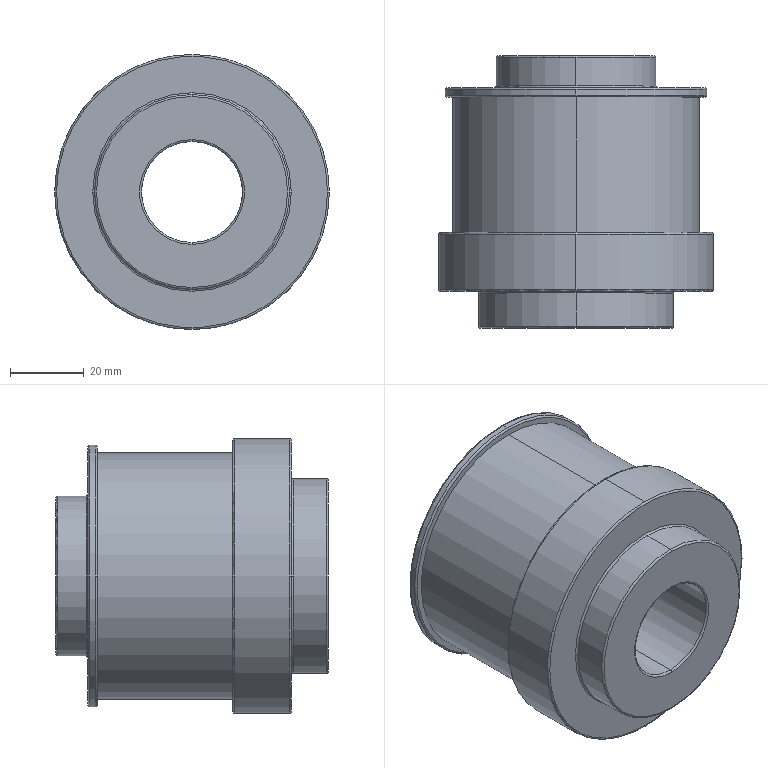Part | SolidWorks | features BaseBody 1 | 1 solid | 38 faces | box 74.696 x 74 x 74.696 mm | volume 200799 mm3 | torus 20 | cylinder 12 | plane 6 | commonest cylinder face diameters 27.5 x2 43.493 x2 52.995 x2 67 x2 71.246 x2 74.696 x2
STEP:
#1=CARTESIAN_POINT('',(1930.753,195.2,853.));
#2=VERTEX_POINT('',#1);
#3=CARTESIAN_POINT('',(1975.247,195.2,853.));
#4=VERTEX_POINT('',#3);
#5=CARTESIAN_POINT('',(1953.,195.2,853.));
#6=DIRECTION('',(0.,-1.,0.));
#7=DIRECTION('',(1.,0.,0.));
#8=AXIS2_PLACEMENT_3D('',#5,#6,#7);
#9=CIRCLE('',#8,22.247);
#10=EDGE_CURVE('',#2,#4,#9,.T.);
#11=ORIENTED_EDGE('',*,*,#10,.F.);
#12=CARTESIAN_POINT('',(1931.253,195.7,853.));
#13=VERTEX_POINT('',#12);
#14=CARTESIAN_POINT('',(1930.753,195.7,853.));
#15=DIRECTION('',(0.,0.,1.));
#16=DIRECTION('',(0.,-1.,0.));
#17=AXIS2_PLACEMENT_3D('',#14,#15,#16);
#18=CIRCLE('',#17,0.5);
#19=EDGE_CURVE('',#2,#13,#18,.T.);
#20=ORIENTED_EDGE('',*,*,#19,.T.);
#21=CARTESIAN_POINT('',(1953.,195.7,831.253));
#22=VERTEX_POINT('',#21);
#23=CARTESIAN_POINT('',(1953.,195.7,853.));
#24=DIRECTION('',(0.,1.,0.));
#25=DIRECTION('',(1.,0.,0.));
#26=AXIS2_PLACEMENT_3D('',#23,#24,#25);
#27=CIRCLE('',#26,21.747);
#28=EDGE_CURVE('',#22,#13,#27,.T.);
#29=ORIENTED_EDGE('',*,*,#28,.F.);
#30=CARTESIAN_POINT('',(1974.747,195.7,853.));
#31=VERTEX_POINT('',#30);
#32=CARTESIAN_POINT('',(1953.,195.7,853.));
#33=DIRECTION('',(0.,1.,0.));
#34=DIRECTION('',(1.,0.,0.));
#35=AXIS2_PLACEMENT_3D('',#32,#33,#34);
#36=CIRCLE('',#35,21.747);
#37=EDGE_CURVE('',#31,#22,#36,.T.);
#38=ORIENTED_EDGE('',*,*,#37,.F.);
#39=CARTESIAN_POINT('',(1975.247,195.7,853.));
#40=DIRECTION('',(0.,0.,-1.));
#41=DIRECTION('',(0.,1.,0.));
#42=AXIS2_PLACEMENT_3D('',#39,#40,#41);
#43=CIRCLE('',#42,0.5);
#44=EDGE_CURVE('',#4,#31,#43,.T.);
#45=ORIENTED_EDGE('',*,*,#44,.F.);
#46=EDGE_LOOP('',(#11,#20,#29,#38,#45));
#47=FACE_OUTER_BOUND('',#46,.T.);
#48=CARTESIAN_POINT('',(1953.,195.7,853.));
#49=DIRECTION('',(0.,-1.,0.));
#50=DIRECTION('',(1.,0.,0.));
#51=AXIS2_PLACEMENT_3D('',#48,#49,#50);
#52=TOROIDAL_SURFACE('',#51,22.247,0.5);
#53=ADVANCED_FACE('',(#47),#52,.F.);
#54=CARTESIAN_POINT('',(1953.,130.4,839.25));
#55=VERTEX_POINT('',#54);
#56=CARTESIAN_POINT('',(1953.,130.4,866.75));
#57=VERTEX_POINT('',#56);
#58=CARTESIAN_POINT('',(1953.,130.4,853.));
#59=DIRECTION('',(0.,-1.,0.));
#60=DIRECTION('',(0.,0.,1.));
#61=AXIS2_PLACEMENT_3D('',#58,#59,#60);
#62=CIRCLE('',#61,13.75);
#63=EDGE_CURVE('',#55,#57,#62,.T.);
#64=ORIENTED_EDGE('',*,*,#63,.F.);
#65=CARTESIAN_POINT('',(1953.,129.9,838.75));
#66=VERTEX_POINT('',#65);
#67=CARTESIAN_POINT('',(1953.,130.4,838.75));
#68=DIRECTION('',(1.,0.,0.));
#69=DIRECTION('',(0.,0.,-1.));
#70=AXIS2_PLACEMENT_3D('',#67,#68,#69);
#71=CIRCLE('',#70,0.5);
#72=EDGE_CURVE('',#55,#66,#71,.T.);
#73=ORIENTED_EDGE('',*,*,#72,.T.);
#74=CARTESIAN_POINT('',(1953.,129.9,867.25));
#75=VERTEX_POINT('',#74);
#76=CARTESIAN_POINT('',(1953.,129.9,853.));
#77=DIRECTION('',(0.,1.,0.));
#78=DIRECTION('',(0.,0.,1.));
#79=AXIS2_PLACEMENT_3D('',#76,#77,#78);
#80=CIRCLE('',#79,14.25);
#81=EDGE_CURVE('',#75,#66,#80,.T.);
#82=ORIENTED_EDGE('',*,*,#81,.F.);
#83=CARTESIAN_POINT('',(1953.,130.4,867.25));
#84=DIRECTION('',(-1.,0.,0.));
#85=DIRECTION('',(0.,0.,1.));
#86=AXIS2_PLACEMENT_3D('',#83,#84,#85);
#87=CIRCLE('',#86,0.5);
#88=EDGE_CURVE('',#57,#75,#87,.T.);
#89=ORIENTED_EDGE('',*,*,#88,.F.);
#90=EDGE_LOOP('',(#64,#73,#82,#89));
#91=FACE_OUTER_BOUND('',#90,.T.);
#92=CARTESIAN_POINT('',(1953.,130.4,853.));
#93=DIRECTION('',(0.,1.,0.));
#94=DIRECTION('',(0.,0.,1.));
#95=AXIS2_PLACEMENT_3D('',#92,#93,#94);
#96=TOROIDAL_SURFACE('',#95,14.25,0.5);
#97=ADVANCED_FACE('',(#91),#96,.T.);
#98=CARTESIAN_POINT('',(1953.,129.9,827.003));
#99=VERTEX_POINT('',#98);
#100=CARTESIAN_POINT('',(1953.,129.9,878.997));
#101=VERTEX_POINT('',#100);
#102=CARTESIAN_POINT('',(1953.,129.9,853.));
#103=DIRECTION('',(0.,-1.,0.));
#104=DIRECTION('',(0.,0.,1.));
#105=AXIS2_PLACEMENT_3D('',#102,#103,#104);
#106=CIRCLE('',#105,25.997);
#107=EDGE_CURVE('',#99,#101,#106,.T.);
#108=ORIENTED_EDGE('',*,*,#107,.F.);
#109=CARTESIAN_POINT('',(1953.,130.4,826.503));
#110=VERTEX_POINT('',#109);
#111=CARTESIAN_POINT('',(1953.,130.4,827.003));
#112=DIRECTION('',(1.,0.,0.));
#113=DIRECTION('',(0.,0.,-1.));
#114=AXIS2_PLACEMENT_3D('',#111,#112,#113);
#115=CIRCLE('',#114,0.5);
#116=EDGE_CURVE('',#99,#110,#115,.T.);
#117=ORIENTED_EDGE('',*,*,#116,.T.);
#118=CARTESIAN_POINT('',(1953.,130.4,879.497));
#119=VERTEX_POINT('',#118);
#120=CARTESIAN_POINT('',(1953.,130.4,853.));
#121=DIRECTION('',(0.,1.,0.));
#122=DIRECTION('',(0.,0.,1.));
#123=AXIS2_PLACEMENT_3D('',#120,#121,#122);
#124=CIRCLE('',#123,26.497);
#125=EDGE_CURVE('',#119,#110,#124,.T.);
#126=ORIENTED_EDGE('',*,*,#125,.F.);
#127=CARTESIAN_POINT('',(1953.,130.4,878.997));
#128=DIRECTION('',(-1.,0.,0.));
#129=DIRECTION('',(0.,0.,1.));
#130=AXIS2_PLACEMENT_3D('',#127,#128,#129);
#131=CIRCLE('',#130,0.5);
#132=EDGE_CURVE('',#101,#119,#131,.T.);
#133=ORIENTED_EDGE('',*,*,#132,.F.);
#134=EDGE_LOOP('',(#108,#117,#126,#133));
#135=FACE_OUTER_BOUND('',#134,.T.);
#136=CARTESIAN_POINT('',(1953.,130.4,853.));
#137=DIRECTION('',(0.,1.,0.));
#138=DIRECTION('',(0.,0.,1.));
#139=AXIS2_PLACEMENT_3D('',#136,#137,#138);
#140=TOROIDAL_SURFACE('',#139,25.997,0.5);
#141=ADVANCED_FACE('',(#135),#140,.T.);
#142=CARTESIAN_POINT('',(1926.503,139.398,853.));
#143=VERTEX_POINT('',#142);
#144=CARTESIAN_POINT('',(1953.,139.398,826.503));
#145=VERTEX_POINT('',#144);
#146=CARTESIAN_POINT('',(1953.,139.398,853.));
#147=DIRECTION('',(0.,-1.,0.));
#148=DIRECTION('',(1.,0.,0.));
#149=AXIS2_PLACEMENT_3D('',#146,#147,#148);
#150=CIRCLE('',#149,26.497);
#151=EDGE_CURVE('',#143,#145,#150,.T.);
#152=ORIENTED_EDGE('',*,*,#151,.F.);
#153=CARTESIAN_POINT('',(1926.003,139.898,853.));
#154=VERTEX_POINT('',#153);
#155=CARTESIAN_POINT('',(1926.003,139.398,853.));
#156=DIRECTION('',(0.,0.,1.));
#157=DIRECTION('',(0.,-1.,0.));
#158=AXIS2_PLACEMENT_3D('',#155,#156,#157);
#159=CIRCLE('',#158,0.5);
#160=EDGE_CURVE('',#143,#154,#159,.T.);
#161=ORIENTED_EDGE('',*,*,#160,.T.);
#162=CARTESIAN_POINT('',(1979.997,139.898,853.));
#163=VERTEX_POINT('',#162);
#164=CARTESIAN_POINT('',(1953.,139.898,853.));
#165=DIRECTION('',(0.,1.,0.));
#166=DIRECTION('',(1.,0.,0.));
#167=AXIS2_PLACEMENT_3D('',#164,#165,#166);
#168=CIRCLE('',#167,26.997);
#169=EDGE_CURVE('',#163,#154,#168,.T.);
#170=ORIENTED_EDGE('',*,*,#169,.F.);
#171=CARTESIAN_POINT('',(1979.497,139.398,853.));
#172=VERTEX_POINT('',#171);
#173=CARTESIAN_POINT('',(1979.997,139.398,853.));
#174=DIRECTION('',(0.,0.,-1.));
#175=DIRECTION('',(0.,1.,0.));
#176=AXIS2_PLACEMENT_3D('',#173,#174,#175);
#177=CIRCLE('',#176,0.5);
#178=EDGE_CURVE('',#172,#163,#177,.T.);
#179=ORIENTED_EDGE('',*,*,#178,.F.);
#180=CARTESIAN_POINT('',(1953.,139.398,853.));
#181=DIRECTION('',(0.,-1.,0.));
#182=DIRECTION('',(1.,0.,0.));
#183=AXIS2_PLACEMENT_3D('',#180,#181,#182);
#184=CIRCLE('',#183,26.497);
#185=EDGE_CURVE('',#145,#172,#184,.T.);
#186=ORIENTED_EDGE('',*,*,#185,.F.);
#187=EDGE_LOOP('',(#152,#161,#170,#179,#186));
#188=FACE_OUTER_BOUND('',#187,.T.);
#189=CARTESIAN_POINT('',(1953.,139.398,853.));
#190=DIRECTION('',(0.,-1.,0.));
#191=DIRECTION('',(1.,0.,0.));
#192=AXIS2_PLACEMENT_3D('',#189,#190,#191);
#193=TOROIDAL_SURFACE('',#192,26.997,0.5);
#194=ADVANCED_FACE('',(#188),#193,.F.);
#195=CARTESIAN_POINT('',(1915.652,140.398,853.));
#196=VERTEX_POINT('',#195);
#197=CARTESIAN_POINT('',(1953.,140.398,890.348));
#198=VERTEX_POINT('',#197);
#199=CARTESIAN_POINT('',(1953.,140.398,853.));
#200=DIRECTION('',(0.,1.,0.));
#201=DIRECTION('',(1.,0.,0.));
#202=AXIS2_PLACEMENT_3D('',#199,#200,#201);
#203=CIRCLE('',#202,37.348);
#204=EDGE_CURVE('',#196,#198,#203,.T.);
#205=ORIENTED_EDGE('',*,*,#204,.F.);
#206=CARTESIAN_POINT('',(1916.152,139.898,853.));
#207=VERTEX_POINT('',#206);
#208=CARTESIAN_POINT('',(1916.152,140.398,853.));
#209=DIRECTION('',(0.,0.,1.));
#210=DIRECTION('',(0.,-1.,0.));
#211=AXIS2_PLACEMENT_3D('',#208,#209,#210);
#212=CIRCLE('',#211,0.5);
#213=EDGE_CURVE('',#196,#207,#212,.T.);
#214=ORIENTED_EDGE('',*,*,#213,.T.);
#215=CARTESIAN_POINT('',(1989.848,139.898,853.));
#216=VERTEX_POINT('',#215);
#217=CARTESIAN_POINT('',(1953.,139.898,853.));
#218=DIRECTION('',(0.,-1.,0.));
#219=DIRECTION('',(1.,0.,0.));
#220=AXIS2_PLACEMENT_3D('',#217,#218,#219);
#221=CIRCLE('',#220,36.848);
#222=EDGE_CURVE('',#216,#207,#221,.T.);
#223=ORIENTED_EDGE('',*,*,#222,.F.);
#224=CARTESIAN_POINT('',(1990.348,140.398,853.));
#225=VERTEX_POINT('',#224);
#226=CARTESIAN_POINT('',(1989.848,140.398,853.));
#227=DIRECTION('',(0.,0.,-1.));
#228=DIRECTION('',(0.,1.,0.));
#229=AXIS2_PLACEMENT_3D('',#226,#227,#228);
#230=CIRCLE('',#229,0.5);
#231=EDGE_CURVE('',#225,#216,#230,.T.);
#232=ORIENTED_EDGE('',*,*,#231,.F.);
#233=CARTESIAN_POINT('',(1953.,140.398,853.));
#234=DIRECTION('',(0.,1.,0.));
#235=DIRECTION('',(1.,0.,0.));
#236=AXIS2_PLACEMENT_3D('',#233,#234,#235);
#237=CIRCLE('',#236,37.348);
#238=EDGE_CURVE('',#198,#225,#237,.T.);
#239=ORIENTED_EDGE('',*,*,#238,.F.);
#240=EDGE_LOOP('',(#205,#214,#223,#232,#239));
#241=FACE_OUTER_BOUND('',#240,.T.);
#242=CARTESIAN_POINT('',(1953.,140.398,853.));
#243=DIRECTION('',(0.,-1.,0.));
#244=DIRECTION('',(1.,0.,0.));
#245=AXIS2_PLACEMENT_3D('',#242,#243,#244);
#246=TOROIDAL_SURFACE('',#245,36.848,0.5);
#247=ADVANCED_FACE('',(#241),#246,.T.);
#248=CARTESIAN_POINT('',(1916.152,155.898,853.));
#249=VERTEX_POINT('',#248);
#250=CARTESIAN_POINT('',(1989.848,155.898,853.));
#251=VERTEX_POINT('',#250);
#252=CARTESIAN_POINT('',(1953.,155.898,853.));
#253=DIRECTION('',(0.,1.,0.));
#254=DIRECTION('',(1.,0.,0.));
#255=AXIS2_PLACEMENT_3D('',#252,#253,#254);
#256=CIRCLE('',#255,36.848);
#257=EDGE_CURVE('',#249,#251,#256,.T.);
#258=ORIENTED_EDGE('',*,*,#257,.F.);
#259=CARTESIAN_POINT('',(1915.652,155.398,853.));
#260=VERTEX_POINT('',#259);
#261=CARTESIAN_POINT('',(1916.152,155.398,853.));
#262=DIRECTION('',(0.,0.,1.));
#263=DIRECTION('',(0.,-1.,0.));
#264=AXIS2_PLACEMENT_3D('',#261,#262,#263);
#265=CIRCLE('',#264,0.5);
#266=EDGE_CURVE('',#249,#260,#265,.T.);
#267=ORIENTED_EDGE('',*,*,#266,.T.);
#268=CARTESIAN_POINT('',(1953.,155.398,890.348));
#269=VERTEX_POINT('',#268);
#270=CARTESIAN_POINT('',(1953.,155.398,853.));
#271=DIRECTION('',(0.,-1.,0.));
#272=DIRECTION('',(1.,0.,0.));
#273=AXIS2_PLACEMENT_3D('',#270,#271,#272);
#274=CIRCLE('',#273,37.348);
#275=EDGE_CURVE('',#269,#260,#274,.T.);
#276=ORIENTED_EDGE('',*,*,#275,.F.);
#277=CARTESIAN_POINT('',(1990.348,155.398,853.));
#278=VERTEX_POINT('',#277);
#279=CARTESIAN_POINT('',(1953.,155.398,853.));
#280=DIRECTION('',(0.,-1.,0.));
#281=DIRECTION('',(1.,0.,0.));
#282=AXIS2_PLACEMENT_3D('',#279,#280,#281);
#283=CIRCLE('',#282,37.348);
#284=EDGE_CURVE('',#278,#269,#283,.T.);
#285=ORIENTED_EDGE('',*,*,#284,.F.);
#286=CARTESIAN_POINT('',(1989.848,155.398,853.));
#287=DIRECTION('',(0.,0.,-1.));
#288=DIRECTION('',(0.,1.,0.));
#289=AXIS2_PLACEMENT_3D('',#286,#287,#288);
#290=CIRCLE('',#289,0.5);
#291=EDGE_CURVE('',#251,#278,#290,.T.);
#292=ORIENTED_EDGE('',*,*,#291,.F.);
#293=EDGE_LOOP('',(#258,#267,#276,#285,#292));
#294=FACE_OUTER_BOUND('',#293,.T.);
#295=CARTESIAN_POINT('',(1953.,155.398,853.));
#296=DIRECTION('',(0.,-1.,0.));
#297=DIRECTION('',(1.,0.,0.));
#298=AXIS2_PLACEMENT_3D('',#295,#296,#297);
#299=TOROIDAL_SURFACE('',#298,36.848,0.5);
#300=ADVANCED_FACE('',(#294),#299,.T.);
#301=CARTESIAN_POINT('',(1917.377,193.2,853.));
#302=VERTEX_POINT('',#301);
#303=CARTESIAN_POINT('',(1953.,193.2,888.623));
#304=VERTEX_POINT('',#303);
#305=CARTESIAN_POINT('',(1953.,193.2,853.));
#306=DIRECTION('',(0.,1.,0.));
#307=DIRECTION('',(1.,0.,0.));
#308=AXIS2_PLACEMENT_3D('',#305,#306,#307);
#309=CIRCLE('',#308,35.623);
#310=EDGE_CURVE('',#302,#304,#309,.T.);
#311=ORIENTED_EDGE('',*,*,#310,.F.);
#312=CARTESIAN_POINT('',(1917.877,192.7,853.));
#313=VERTEX_POINT('',#312);
#314=CARTESIAN_POINT('',(1917.877,193.2,853.));
#315=DIRECTION('',(0.,0.,1.));
#316=DIRECTION('',(0.,-1.,0.));
#317=AXIS2_PLACEMENT_3D('',#314,#315,#316);
#318=CIRCLE('',#317,0.5);
#319=EDGE_CURVE('',#302,#313,#318,.T.);
#320=ORIENTED_EDGE('',*,*,#319,.T.);
#321=CARTESIAN_POINT('',(1988.123,192.7,853.));
#322=VERTEX_POINT('',#321);
#323=CARTESIAN_POINT('',(1953.,192.7,853.));
#324=DIRECTION('',(0.,-1.,0.));
#325=DIRECTION('',(1.,0.,0.));
#326=AXIS2_PLACEMENT_3D('',#323,#324,#325);
#327=CIRCLE('',#326,35.123);
#328=EDGE_CURVE('',#322,#313,#327,.T.);
#329=ORIENTED_EDGE('',*,*,#328,.F.);
#330=CARTESIAN_POINT('',(1988.623,193.2,853.));
#331=VERTEX_POINT('',#330);
#332=CARTESIAN_POINT('',(1988.123,193.2,853.));
#333=DIRECTION('',(0.,0.,-1.));
#334=DIRECTION('',(0.,1.,0.));
#335=AXIS2_PLACEMENT_3D('',#332,#333,#334);
#336=CIRCLE('',#335,0.5);
#337=EDGE_CURVE('',#331,#322,#336,.T.);
#338=ORIENTED_EDGE('',*,*,#337,.F.);
#339=CARTESIAN_POINT('',(1953.,193.2,853.));
#340=DIRECTION('',(0.,1.,0.));
#341=DIRECTION('',(1.,0.,0.));
#342=AXIS2_PLACEMENT_3D('',#339,#340,#341);
#343=CIRCLE('',#342,35.623);
#344=EDGE_CURVE('',#304,#331,#343,.T.);
#345=ORIENTED_EDGE('',*,*,#344,.F.);
#346=EDGE_LOOP('',(#311,#320,#329,#338,#345));
#347=FACE_OUTER_BOUND('',#346,.T.);
#348=CARTESIAN_POINT('',(1953.,193.2,853.));
#349=DIRECTION('',(0.,-1.,0.));
#350=DIRECTION('',(1.,0.,0.));
#351=AXIS2_PLACEMENT_3D('',#348,#349,#350);
#352=TOROIDAL_SURFACE('',#351,35.123,0.5);
#353=ADVANCED_FACE('',(#347),#352,.T.);
#354=CARTESIAN_POINT('',(1917.877,195.2,853.));
#355=VERTEX_POINT('',#354);
#356=CARTESIAN_POINT('',(1988.123,195.2,853.));
#357=VERTEX_POINT('',#356);
#358=CARTESIAN_POINT('',(1953.,195.2,853.));
#359=DIRECTION('',(0.,1.,0.));
#360=DIRECTION('',(1.,0.,0.));
#361=AXIS2_PLACEMENT_3D('',#358,#359,#360);
#362=CIRCLE('',#361,35.123);
#363=EDGE_CURVE('',#355,#357,#362,.T.);
#364=ORIENTED_EDGE('',*,*,#363,.F.);
#365=CARTESIAN_POINT('',(1917.377,194.7,853.));
#366=VERTEX_POINT('',#365);
#367=CARTESIAN_POINT('',(1917.877,194.7,853.));
#368=DIRECTION('',(0.,0.,1.));
#369=DIRECTION('',(0.,-1.,0.));
#370=AXIS2_PLACEMENT_3D('',#367,#368,#369);
#371=CIRCLE('',#370,0.5);
#372=EDGE_CURVE('',#355,#366,#371,.T.);
#373=ORIENTED_EDGE('',*,*,#372,.T.);
#374=CARTESIAN_POINT('',(1953.,194.7,888.623));
#375=VERTEX_POINT('',#374);
#376=CARTESIAN_POINT('',(1953.,194.7,853.));
#377=DIRECTION('',(0.,-1.,0.));
#378=DIRECTION('',(1.,0.,0.));
#379=AXIS2_PLACEMENT_3D('',#376,#377,#378);
#380=CIRCLE('',#379,35.623);
#381=EDGE_CURVE('',#375,#366,#380,.T.);
#382=ORIENTED_EDGE('',*,*,#381,.F.);
#383=CARTESIAN_POINT('',(1988.623,194.7,853.));
#384=VERTEX_POINT('',#383);
#385=CARTESIAN_POINT('',(1953.,194.7,853.));
#386=DIRECTION('',(0.,-1.,0.));
#387=DIRECTION('',(1.,0.,0.));
#388=AXIS2_PLACEMENT_3D('',#385,#386,#387);
#389=CIRCLE('',#388,35.623);
#390=EDGE_CURVE('',#384,#375,#389,.T.);
#391=ORIENTED_EDGE('',*,*,#390,.F.);
#392=CARTESIAN_POINT('',(1988.123,194.7,853.));
#393=DIRECTION('',(0.,0.,-1.));
#394=DIRECTION('',(0.,1.,0.));
#395=AXIS2_PLACEMENT_3D('',#392,#393,#394);
#396=CIRCLE('',#395,0.5);
#397=EDGE_CURVE('',#357,#384,#396,.T.);
#398=ORIENTED_EDGE('',*,*,#397,.F.);
#399=EDGE_LOOP('',(#364,#373,#382,#391,#398));
#400=FACE_OUTER_BOUND('',#399,.T.);
#401=CARTESIAN_POINT('',(1953.,194.7,853.));
#402=DIRECTION('',(0.,-1.,0.));
#403=DIRECTION('',(1.,0.,0.));
#404=AXIS2_PLACEMENT_3D('',#401,#402,#403);
#405=TOROIDAL_SURFACE('',#404,35.123,0.5);
#406=ADVANCED_FACE('',(#400),#405,.T.);
#407=CARTESIAN_POINT('',(1939.25,203.4,853.));
#408=VERTEX_POINT('',#407);
#409=CARTESIAN_POINT('',(1953.,203.4,866.75));
#410=VERTEX_POINT('',#409);
#411=CARTESIAN_POINT('',(1953.,203.4,853.));
#412=DIRECTION('',(0.,1.,0.));
#413=DIRECTION('',(1.,0.,0.));
#414=AXIS2_PLACEMENT_3D('',#411,#412,#413);
#415=CIRCLE('',#414,13.75);
#416=EDGE_CURVE('',#408,#410,#415,.T.);
#417=ORIENTED_EDGE('',*,*,#416,.F.);
#418=CARTESIAN_POINT('',(1938.75,203.9,853.));
#419=VERTEX_POINT('',#418);
#420=CARTESIAN_POINT('',(1938.75,203.4,853.));
#421=DIRECTION('',(0.,0.,1.));
#422=DIRECTION('',(0.,-1.,0.));
#423=AXIS2_PLACEMENT_3D('',#420,#421,#422);
#424=CIRCLE('',#423,0.5);
#425=EDGE_CURVE('',#408,#419,#424,.T.);
#426=ORIENTED_EDGE('',*,*,#425,.T.);
#427=CARTESIAN_POINT('',(1967.25,203.9,853.));
#428=VERTEX_POINT('',#427);
#429=CARTESIAN_POINT('',(1953.,203.9,853.));
#430=DIRECTION('',(0.,-1.,0.));
#431=DIRECTION('',(1.,0.,0.));
#432=AXIS2_PLACEMENT_3D('',#429,#430,#431);
#433=CIRCLE('',#432,14.25);
#434=EDGE_CURVE('',#428,#419,#433,.T.);
#435=ORIENTED_EDGE('',*,*,#434,.F.);
#436=CARTESIAN_POINT('',(1966.75,203.4,853.));
#437=VERTEX_POINT('',#436);
#438=CARTESIAN_POINT('',(1967.25,203.4,853.));
#439=DIRECTION('',(0.,0.,-1.));
#440=DIRECTION('',(0.,1.,0.));
#441=AXIS2_PLACEMENT_3D('',#438,#439,#440);
#442=CIRCLE('',#441,0.5);
#443=EDGE_CURVE('',#437,#428,#442,.T.);
#444=ORIENTED_EDGE('',*,*,#443,.F.);
#445=CARTESIAN_POINT('',(1953.,203.4,853.));
#446=DIRECTION('',(0.,1.,0.));
#447=DIRECTION('',(1.,0.,0.));
#448=AXIS2_PLACEMENT_3D('',#445,#446,#447);
#449=CIRCLE('',#448,13.75);
#450=EDGE_CURVE('',#410,#437,#449,.T.);
#451=ORIENTED_EDGE('',*,*,#450,.F.);
#452=EDGE_LOOP('',(#417,#426,#435,#444,#451));
#453=FACE_OUTER_BOUND('',#452,.T.);
#454=CARTESIAN_POINT('',(1953.,203.4,853.));
#455=DIRECTION('',(0.,-1.,0.));
#456=DIRECTION('',(1.,0.,0.));
#457=AXIS2_PLACEMENT_3D('',#454,#455,#456);
#458=TOROIDAL_SURFACE('',#457,14.25,0.5);
#459=ADVANCED_FACE('',(#453),#458,.T.);
#460=CARTESIAN_POINT('',(1931.753,203.9,853.));
#461=VERTEX_POINT('',#460);
#462=CARTESIAN_POINT('',(1974.247,203.9,853.));
#463=VERTEX_POINT('',#462);
#464=CARTESIAN_POINT('',(1953.,203.9,853.));
#465=DIRECTION('',(0.,1.,0.));
#466=DIRECTION('',(1.,0.,0.));
#467=AXIS2_PLACEMENT_3D('',#464,#465,#466);
#468=CIRCLE('',#467,21.247);
#469=EDGE_CURVE('',#461,#463,#468,.T.);
#470=ORIENTED_EDGE('',*,*,#469,.F.);
#471=CARTESIAN_POINT('',(1931.253,203.4,853.));
#472=VERTEX_POINT('',#471);
#473=CARTESIAN_POINT('',(1931.753,203.4,853.));
#474=DIRECTION('',(0.,0.,1.));
#475=DIRECTION('',(0.,-1.,0.));
#476=AXIS2_PLACEMENT_3D('',#473,#474,#475);
#477=CIRCLE('',#476,0.5);
#478=EDGE_CURVE('',#461,#472,#477,.T.);
#479=ORIENTED_EDGE('',*,*,#478,.T.);
#480=CARTESIAN_POINT('',(1953.,203.4,874.747));
#481=VERTEX_POINT('',#480);
#482=CARTESIAN_POINT('',(1953.,203.4,853.));
#483=DIRECTION('',(0.,-1.,0.));
#484=DIRECTION('',(1.,0.,0.));
#485=AXIS2_PLACEMENT_3D('',#482,#483,#484);
#486=CIRCLE('',#485,21.747);
#487=EDGE_CURVE('',#481,#472,#486,.T.);
#488=ORIENTED_EDGE('',*,*,#487,.F.);
#489=CARTESIAN_POINT('',(1974.747,203.4,853.));
#490=VERTEX_POINT('',#489);
#491=CARTESIAN_POINT('',(1953.,203.4,853.));
#492=DIRECTION('',(0.,-1.,0.));
#493=DIRECTION('',(1.,0.,0.));
#494=AXIS2_PLACEMENT_3D('',#491,#492,#493);
#495=CIRCLE('',#494,21.747);
#496=EDGE_CURVE('',#490,#481,#495,.T.);
#497=ORIENTED_EDGE('',*,*,#496,.F.);
#498=CARTESIAN_POINT('',(1974.247,203.4,853.));
#499=DIRECTION('',(0.,0.,-1.));
#500=DIRECTION('',(0.,1.,0.));
#501=AXIS2_PLACEMENT_3D('',#498,#499,#500);
#502=CIRCLE('',#501,0.5);
#503=EDGE_CURVE('',#463,#490,#502,.T.);
#504=ORIENTED_EDGE('',*,*,#503,.F.);
#505=EDGE_LOOP('',(#470,#479,#488,#497,#504));
#506=FACE_OUTER_BOUND('',#505,.T.);
#507=CARTESIAN_POINT('',(1953.,203.4,853.));
#508=DIRECTION('',(0.,-1.,0.));
#509=DIRECTION('',(1.,0.,0.));
#510=AXIS2_PLACEMENT_3D('',#507,#508,#509);
#511=TOROIDAL_SURFACE('',#510,21.247,0.5);
#512=ADVANCED_FACE('',(#506),#511,.T.);
#513=CARTESIAN_POINT('',(1953.,203.4,839.25));
#514=VERTEX_POINT('',#513);
#515=CARTESIAN_POINT('',(1953.,203.4,853.));
#516=DIRECTION('',(0.,1.,0.));
#517=DIRECTION('',(1.,0.,0.));
#518=AXIS2_PLACEMENT_3D('',#515,#516,#517);
#519=CIRCLE('',#518,13.75);
#520=EDGE_CURVE('',#514,#408,#519,.T.);
#521=ORIENTED_EDGE('',*,*,#520,.T.);
#522=ORIENTED_EDGE('',*,*,#416,.T.);
#523=CARTESIAN_POINT('',(1953.,217.7,866.75));
#524=DIRECTION('',(0.,-1.,0.));
#525=VECTOR('',#524,1000.);
#526=LINE('',#523,#525);
#527=EDGE_CURVE('',#410,#57,#526,.T.);
#528=ORIENTED_EDGE('',*,*,#527,.T.);
#529=CARTESIAN_POINT('',(1953.,130.4,853.));
#530=DIRECTION('',(0.,-1.,0.));
#531=DIRECTION('',(0.,0.,1.));
#532=AXIS2_PLACEMENT_3D('',#529,#530,#531);
#533=CIRCLE('',#532,13.75);
#534=EDGE_CURVE('',#57,#55,#533,.T.);
#535=ORIENTED_EDGE('',*,*,#534,.T.);
#536=CARTESIAN_POINT('',(1953.,217.7,839.25));
#537=DIRECTION('',(0.,-1.,0.));
#538=VECTOR('',#537,1000.);
#539=LINE('',#536,#538);
#540=EDGE_CURVE('',#514,#55,#539,.T.);
#541=ORIENTED_EDGE('',*,*,#540,.F.);
#542=EDGE_LOOP('',(#521,#522,#528,#535,#541));
#543=FACE_OUTER_BOUND('',#542,.T.);
#544=CARTESIAN_POINT('',(1953.,217.7,853.));
#545=DIRECTION('',(0.,-1.,0.));
#546=DIRECTION('',(0.,0.,-1.));
#547=AXIS2_PLACEMENT_3D('',#544,#545,#546);
#548=CYLINDRICAL_SURFACE('',#547,13.75);
#549=ADVANCED_FACE('',(#543),#548,.F.);
#550=ORIENTED_EDGE('',*,*,#125,.T.);
#551=CARTESIAN_POINT('',(1953.,129.9,826.503));
#552=DIRECTION('',(0.,1.,0.));
#553=VECTOR('',#552,1000.);
#554=LINE('',#551,#553);
#555=EDGE_CURVE('',#110,#145,#554,.T.);
#556=ORIENTED_EDGE('',*,*,#555,.T.);
#557=ORIENTED_EDGE('',*,*,#185,.T.);
#558=CARTESIAN_POINT('',(1953.,139.398,879.497));
#559=VERTEX_POINT('',#558);
#560=CARTESIAN_POINT('',(1953.,139.398,853.));
#561=DIRECTION('',(0.,-1.,0.));
#562=DIRECTION('',(1.,0.,0.));
#563=AXIS2_PLACEMENT_3D('',#560,#561,#562);
#564=CIRCLE('',#563,26.497);
#565=EDGE_CURVE('',#172,#559,#564,.T.);
#566=ORIENTED_EDGE('',*,*,#565,.T.);
#567=CARTESIAN_POINT('',(1953.,129.9,879.497));
#568=DIRECTION('',(0.,1.,0.));
#569=VECTOR('',#568,1000.);
#570=LINE('',#567,#569);
#571=EDGE_CURVE('',#119,#559,#570,.T.);
#572=ORIENTED_EDGE('',*,*,#571,.F.);
#573=EDGE_LOOP('',(#550,#556,#557,#566,#572));
#574=FACE_OUTER_BOUND('',#573,.T.);
#575=CARTESIAN_POINT('',(1953.,129.9,853.));
#576=DIRECTION('',(0.,1.,0.));
#577=DIRECTION('',(0.,0.,1.));
#578=AXIS2_PLACEMENT_3D('',#575,#576,#577);
#579=CYLINDRICAL_SURFACE('',#578,26.497);
#580=ADVANCED_FACE('',(#574),#579,.T.);
#581=CARTESIAN_POINT('',(1953.,155.398,815.652));
#582=VERTEX_POINT('',#581);
#583=CARTESIAN_POINT('',(1953.,155.398,853.));
#584=DIRECTION('',(0.,-1.,0.));
#585=DIRECTION('',(1.,0.,0.));
#586=AXIS2_PLACEMENT_3D('',#583,#584,#585);
#587=CIRCLE('',#586,37.348);
#588=EDGE_CURVE('',#582,#278,#587,.T.);
#589=ORIENTED_EDGE('',*,*,#588,.T.);
#590=ORIENTED_EDGE('',*,*,#284,.T.);
#591=CARTESIAN_POINT('',(1953.,155.898,890.348));
#592=DIRECTION('',(0.,-1.,0.));
#593=VECTOR('',#592,1000.);
#594=LINE('',#591,#593);
#595=EDGE_CURVE('',#269,#198,#594,.T.);
#596=ORIENTED_EDGE('',*,*,#595,.T.);
#597=ORIENTED_EDGE('',*,*,#238,.T.);
#598=CARTESIAN_POINT('',(1953.,140.398,815.652));
#599=VERTEX_POINT('',#598);
#600=CARTESIAN_POINT('',(1953.,140.398,853.));
#601=DIRECTION('',(0.,1.,0.));
#602=DIRECTION('',(1.,0.,0.));
#603=AXIS2_PLACEMENT_3D('',#600,#601,#602);
#604=CIRCLE('',#603,37.348);
#605=EDGE_CURVE('',#225,#599,#604,.T.);
#606=ORIENTED_EDGE('',*,*,#605,.T.);
#607=CARTESIAN_POINT('',(1953.,155.898,815.652));
#608=DIRECTION('',(0.,-1.,0.));
#609=VECTOR('',#608,1000.);
#610=LINE('',#607,#609);
#611=EDGE_CURVE('',#582,#599,#610,.T.);
#612=ORIENTED_EDGE('',*,*,#611,.F.);
#613=EDGE_LOOP('',(#589,#590,#596,#597,#606,#612));
#614=FACE_OUTER_BOUND('',#613,.T.);
#615=CARTESIAN_POINT('',(1953.,155.898,853.));
#616=DIRECTION('',(0.,-1.,0.));
#617=DIRECTION('',(0.,0.,-1.));
#618=AXIS2_PLACEMENT_3D('',#615,#616,#617);
#619=CYLINDRICAL_SURFACE('',#618,37.348);
#620=ADVANCED_FACE('',(#614),#619,.T.);
#621=CARTESIAN_POINT('',(1953.,155.898,886.5));
#622=VERTEX_POINT('',#621);
#623=CARTESIAN_POINT('',(1953.,155.898,819.5));
#624=VERTEX_POINT('',#623);
#625=CARTESIAN_POINT('',(1953.,155.898,853.));
#626=DIRECTION('',(0.,1.,0.));
#627=DIRECTION('',(0.,0.,-1.));
#628=AXIS2_PLACEMENT_3D('',#625,#626,#627);
#629=CIRCLE('',#628,33.5);
#630=EDGE_CURVE('',#622,#624,#629,.T.);
#631=ORIENTED_EDGE('',*,*,#630,.T.);
#632=CARTESIAN_POINT('',(1953.,192.7,819.5));
#633=VERTEX_POINT('',#632);
#634=CARTESIAN_POINT('',(1953.,155.,819.5));
#635=DIRECTION('',(0.,1.,0.));
#636=VECTOR('',#635,1000.);
#637=LINE('',#634,#636);
#638=EDGE_CURVE('',#624,#633,#637,.T.);
#639=ORIENTED_EDGE('',*,*,#638,.T.);
#640=CARTESIAN_POINT('',(1953.,192.7,886.5));
#641=VERTEX_POINT('',#640);
#642=CARTESIAN_POINT('',(1953.,192.7,853.));
#643=DIRECTION('',(0.,-1.,0.));
#644=DIRECTION('',(0.,0.,1.));
#645=AXIS2_PLACEMENT_3D('',#642,#643,#644);
#646=CIRCLE('',#645,33.5);
#647=EDGE_CURVE('',#633,#641,#646,.T.);
#648=ORIENTED_EDGE('',*,*,#647,.T.);
#649=CARTESIAN_POINT('',(1953.,155.,886.5));
#650=DIRECTION('',(0.,1.,0.));
#651=VECTOR('',#650,1000.);
#652=LINE('',#649,#651);
#653=EDGE_CURVE('',#622,#641,#652,.T.);
#654=ORIENTED_EDGE('',*,*,#653,.F.);
#655=EDGE_LOOP('',(#631,#639,#648,#654));
#656=FACE_OUTER_BOUND('',#655,.T.);
#657=CARTESIAN_POINT('',(1953.,155.,853.));
#658=DIRECTION('',(0.,1.,0.));
#659=DIRECTION('',(0.,0.,1.));
#660=AXIS2_PLACEMENT_3D('',#657,#658,#659);
#661=CYLINDRICAL_SURFACE('',#660,33.5);
#662=ADVANCED_FACE('',(#656),#661,.T.);
#663=ORIENTED_EDGE('',*,*,#344,.T.);
#664=CARTESIAN_POINT('',(1953.,193.2,817.377));
#665=VERTEX_POINT('',#664);
#666=CARTESIAN_POINT('',(1953.,193.2,853.));
#667=DIRECTION('',(0.,1.,0.));
#668=DIRECTION('',(1.,0.,0.));
#669=AXIS2_PLACEMENT_3D('',#666,#667,#668);
#670=CIRCLE('',#669,35.623);
#671=EDGE_CURVE('',#331,#665,#670,.T.);
#672=ORIENTED_EDGE('',*,*,#671,.T.);
#673=CARTESIAN_POINT('',(1953.,194.7,817.377));
#674=VERTEX_POINT('',#673);
#675=CARTESIAN_POINT('',(1953.,192.7,817.377));
#676=DIRECTION('',(0.,1.,0.));
#677=VECTOR('',#676,1000.);
#678=LINE('',#675,#677);
#679=EDGE_CURVE('',#665,#674,#678,.T.);
#680=ORIENTED_EDGE('',*,*,#679,.T.);
#681=CARTESIAN_POINT('',(1953.,194.7,853.));
#682=DIRECTION('',(0.,-1.,0.));
#683=DIRECTION('',(1.,0.,0.));
#684=AXIS2_PLACEMENT_3D('',#681,#682,#683);
#685=CIRCLE('',#684,35.623);
#686=EDGE_CURVE('',#674,#384,#685,.T.);
#687=ORIENTED_EDGE('',*,*,#686,.T.);
#688=ORIENTED_EDGE('',*,*,#390,.T.);
#689=CARTESIAN_POINT('',(1953.,192.7,888.623));
#690=DIRECTION('',(0.,1.,0.));
#691=VECTOR('',#690,1000.);
#692=LINE('',#689,#691);
#693=EDGE_CURVE('',#304,#375,#692,.T.);
#694=ORIENTED_EDGE('',*,*,#693,.F.);
#695=EDGE_LOOP('',(#663,#672,#680,#687,#688,#694));
#696=FACE_OUTER_BOUND('',#695,.T.);
#697=CARTESIAN_POINT('',(1953.,192.7,853.));
#698=DIRECTION('',(0.,1.,0.));
#699=DIRECTION('',(0.,0.,1.));
#700=AXIS2_PLACEMENT_3D('',#697,#698,#699);
#701=CYLINDRICAL_SURFACE('',#700,35.623);
#702=ADVANCED_FACE('',(#696),#701,.T.);
#703=CARTESIAN_POINT('',(1953.,203.4,831.253));
#704=VERTEX_POINT('',#703);
#705=CARTESIAN_POINT('',(1953.,203.4,853.));
#706=DIRECTION('',(0.,-1.,0.));
#707=DIRECTION('',(1.,0.,0.));
#708=AXIS2_PLACEMENT_3D('',#705,#706,#707);
#709=CIRCLE('',#708,21.747);
#710=EDGE_CURVE('',#704,#490,#709,.T.);
#711=ORIENTED_EDGE('',*,*,#710,.T.);
#712=ORIENTED_EDGE('',*,*,#496,.T.);
#713=CARTESIAN_POINT('',(1953.,195.7,874.747));
#714=VERTEX_POINT('',#713);
#715=CARTESIAN_POINT('',(1953.,203.9,874.747));
#716=DIRECTION('',(0.,-1.,0.));
#717=VECTOR('',#716,1000.);
#718=LINE('',#715,#717);
#719=EDGE_CURVE('',#481,#714,#718,.T.);
#720=ORIENTED_EDGE('',*,*,#719,.T.);
#721=CARTESIAN_POINT('',(1953.,195.7,853.));
#722=DIRECTION('',(0.,1.,0.));
#723=DIRECTION('',(1.,0.,0.));
#724=AXIS2_PLACEMENT_3D('',#721,#722,#723);
#725=CIRCLE('',#724,21.747);
#726=EDGE_CURVE('',#714,#31,#725,.T.);
#727=ORIENTED_EDGE('',*,*,#726,.T.);
#728=ORIENTED_EDGE('',*,*,#37,.T.);
#729=CARTESIAN_POINT('',(1953.,203.9,831.253));
#730=DIRECTION('',(0.,-1.,0.));
#731=VECTOR('',#730,1000.);
#732=LINE('',#729,#731);
#733=EDGE_CURVE('',#704,#22,#732,.T.);
#734=ORIENTED_EDGE('',*,*,#733,.F.);
#735=EDGE_LOOP('',(#711,#712,#720,#727,#728,#734));
#736=FACE_OUTER_BOUND('',#735,.T.);
#737=CARTESIAN_POINT('',(1953.,203.9,853.));
#738=DIRECTION('',(0.,-1.,0.));
#739=DIRECTION('',(0.,0.,-1.));
#740=AXIS2_PLACEMENT_3D('',#737,#738,#739);
#741=CYLINDRICAL_SURFACE('',#740,21.747);
#742=ADVANCED_FACE('',(#736),#741,.T.);
#743=ORIENTED_EDGE('',*,*,#434,.T.);
#744=CARTESIAN_POINT('',(1953.,203.9,853.));
#745=DIRECTION('',(0.,-1.,0.));
#746=DIRECTION('',(1.,0.,0.));
#747=AXIS2_PLACEMENT_3D('',#744,#745,#746);
#748=CIRCLE('',#747,14.25);
#749=EDGE_CURVE('',#419,#428,#748,.T.);
#750=ORIENTED_EDGE('',*,*,#749,.T.);
#751=EDGE_LOOP('',(#743,#750));
#752=FACE_BOUND('',#751,.T.);
#753=CARTESIAN_POINT('',(1953.,203.9,853.));
#754=DIRECTION('',(0.,1.,0.));
#755=DIRECTION('',(1.,0.,0.));
#756=AXIS2_PLACEMENT_3D('',#753,#754,#755);
#757=CIRCLE('',#756,21.247);
#758=EDGE_CURVE('',#463,#461,#757,.T.);
#759=ORIENTED_EDGE('',*,*,#758,.T.);
#760=ORIENTED_EDGE('',*,*,#469,.T.);
#761=EDGE_LOOP('',(#759,#760));
#762=FACE_OUTER_BOUND('',#761,.T.);
#763=CARTESIAN_POINT('',(1953.,203.9,853.));
#764=DIRECTION('',(0.,-1.,0.));
#765=DIRECTION('',(1.,0.,0.));
#766=AXIS2_PLACEMENT_3D('',#763,#764,#765);
#767=PLANE('',#766);
#768=ADVANCED_FACE('',(#752,#762),#767,.F.);
#769=ORIENTED_EDGE('',*,*,#81,.T.);
#770=CARTESIAN_POINT('',(1953.,129.9,853.));
#771=DIRECTION('',(0.,1.,0.));
#772=DIRECTION('',(0.,0.,1.));
#773=AXIS2_PLACEMENT_3D('',#770,#771,#772);
#774=CIRCLE('',#773,14.25);
#775=EDGE_CURVE('',#66,#75,#774,.T.);
#776=ORIENTED_EDGE('',*,*,#775,.T.);
#777=EDGE_LOOP('',(#769,#776));
#778=FACE_BOUND('',#777,.T.);
#779=CARTESIAN_POINT('',(1953.,129.9,853.));
#780=DIRECTION('',(0.,-1.,0.));
#781=DIRECTION('',(0.,0.,1.));
#782=AXIS2_PLACEMENT_3D('',#779,#780,#781);
#783=CIRCLE('',#782,25.997);
#784=EDGE_CURVE('',#101,#99,#783,.T.);
#785=ORIENTED_EDGE('',*,*,#784,.T.);
#786=ORIENTED_EDGE('',*,*,#107,.T.);
#787=EDGE_LOOP('',(#785,#786));
#788=FACE_OUTER_BOUND('',#787,.T.);
#789=CARTESIAN_POINT('',(1953.,129.9,853.));
#790=DIRECTION('',(0.,1.,0.));
#791=DIRECTION('',(0.,0.,1.));
#792=AXIS2_PLACEMENT_3D('',#789,#790,#791);
#793=PLANE('',#792);
#794=ADVANCED_FACE('',(#778,#788),#793,.F.);
#795=ORIENTED_EDGE('',*,*,#719,.F.);
#796=ORIENTED_EDGE('',*,*,#487,.T.);
#797=CARTESIAN_POINT('',(1953.,203.4,853.));
#798=DIRECTION('',(0.,-1.,0.));
#799=DIRECTION('',(1.,0.,0.));
#800=AXIS2_PLACEMENT_3D('',#797,#798,#799);
#801=CIRCLE('',#800,21.747);
#802=EDGE_CURVE('',#472,#704,#801,.T.);
#803=ORIENTED_EDGE('',*,*,#802,.T.);
#804=ORIENTED_EDGE('',*,*,#733,.T.);
#805=ORIENTED_EDGE('',*,*,#28,.T.);
#806=CARTESIAN_POINT('',(1953.,195.7,853.));
#807=DIRECTION('',(0.,1.,0.));
#808=DIRECTION('',(1.,0.,0.));
#809=AXIS2_PLACEMENT_3D('',#806,#807,#808);
#810=CIRCLE('',#809,21.747);
#811=EDGE_CURVE('',#13,#714,#810,.T.);
#812=ORIENTED_EDGE('',*,*,#811,.T.);
#813=EDGE_LOOP('',(#795,#796,#803,#804,#805,#812));
#814=FACE_OUTER_BOUND('',#813,.T.);
#815=CARTESIAN_POINT('',(1953.,203.9,853.));
#816=DIRECTION('',(0.,-1.,0.));
#817=DIRECTION('',(0.,0.,-1.));
#818=AXIS2_PLACEMENT_3D('',#815,#816,#817);
#819=CYLINDRICAL_SURFACE('',#818,21.747);
#820=ADVANCED_FACE('',(#814),#819,.T.);
#821=ORIENTED_EDGE('',*,*,#679,.F.);
#822=CARTESIAN_POINT('',(1953.,193.2,853.));
#823=DIRECTION('',(0.,1.,0.));
#824=DIRECTION('',(1.,0.,0.));
#825=AXIS2_PLACEMENT_3D('',#822,#823,#824);
#826=CIRCLE('',#825,35.623);
#827=EDGE_CURVE('',#665,#302,#826,.T.);
#828=ORIENTED_EDGE('',*,*,#827,.T.);
#829=ORIENTED_EDGE('',*,*,#310,.T.);
#830=ORIENTED_EDGE('',*,*,#693,.T.);
#831=ORIENTED_EDGE('',*,*,#381,.T.);
#832=CARTESIAN_POINT('',(1953.,194.7,853.));
#833=DIRECTION('',(0.,-1.,0.));
#834=DIRECTION('',(1.,0.,0.));
#835=AXIS2_PLACEMENT_3D('',#832,#833,#834);
#836=CIRCLE('',#835,35.623);
#837=EDGE_CURVE('',#366,#674,#836,.T.);
#838=ORIENTED_EDGE('',*,*,#837,.T.);
#839=EDGE_LOOP('',(#821,#828,#829,#830,#831,#838));
#840=FACE_OUTER_BOUND('',#839,.T.);
#841=CARTESIAN_POINT('',(1953.,192.7,853.));
#842=DIRECTION('',(0.,1.,0.));
#843=DIRECTION('',(0.,0.,1.));
#844=AXIS2_PLACEMENT_3D('',#841,#842,#843);
#845=CYLINDRICAL_SURFACE('',#844,35.623);
#846=ADVANCED_FACE('',(#840),#845,.T.);
#847=ORIENTED_EDGE('',*,*,#328,.T.);
#848=CARTESIAN_POINT('',(1953.,192.7,853.));
#849=DIRECTION('',(0.,-1.,0.));
#850=DIRECTION('',(1.,0.,0.));
#851=AXIS2_PLACEMENT_3D('',#848,#849,#850);
#852=CIRCLE('',#851,35.123);
#853=EDGE_CURVE('',#313,#322,#852,.T.);
#854=ORIENTED_EDGE('',*,*,#853,.T.);
#855=EDGE_LOOP('',(#847,#854));
#856=FACE_OUTER_BOUND('',#855,.T.);
#857=CARTESIAN_POINT('',(1953.,192.7,853.));
#858=DIRECTION('',(0.,-1.,0.));
#859=DIRECTION('',(0.,0.,1.));
#860=AXIS2_PLACEMENT_3D('',#857,#858,#859);
#861=CIRCLE('',#860,33.5);
#862=EDGE_CURVE('',#641,#633,#861,.T.);
#863=ORIENTED_EDGE('',*,*,#862,.F.);
#864=ORIENTED_EDGE('',*,*,#647,.F.);
#865=EDGE_LOOP('',(#863,#864));
#866=FACE_BOUND('',#865,.T.);
#867=CARTESIAN_POINT('',(1953.,192.7,853.));
#868=DIRECTION('',(0.,-1.,0.));
#869=DIRECTION('',(1.,0.,0.));
#870=AXIS2_PLACEMENT_3D('',#867,#868,#869);
#871=PLANE('',#870);
#872=ADVANCED_FACE('',(#856,#866),#871,.T.);
#873=CARTESIAN_POINT('',(1953.,195.2,853.));
#874=DIRECTION('',(0.,-1.,0.));
#875=DIRECTION('',(1.,0.,0.));
#876=AXIS2_PLACEMENT_3D('',#873,#874,#875);
#877=CIRCLE('',#876,22.247);
#878=EDGE_CURVE('',#4,#2,#877,.T.);
#879=ORIENTED_EDGE('',*,*,#878,.T.);
#880=ORIENTED_EDGE('',*,*,#10,.T.);
#881=EDGE_LOOP('',(#879,#880));
#882=FACE_BOUND('',#881,.T.);
#883=CARTESIAN_POINT('',(1953.,195.2,853.));
#884=DIRECTION('',(0.,1.,0.));
#885=DIRECTION('',(1.,0.,0.));
#886=AXIS2_PLACEMENT_3D('',#883,#884,#885);
#887=CIRCLE('',#886,35.123);
#888=EDGE_CURVE('',#357,#355,#887,.T.);
#889=ORIENTED_EDGE('',*,*,#888,.T.);
#890=ORIENTED_EDGE('',*,*,#363,.T.);
#891=EDGE_LOOP('',(#889,#890));
#892=FACE_OUTER_BOUND('',#891,.T.);
#893=CARTESIAN_POINT('',(1953.,195.2,853.));
#894=DIRECTION('',(0.,-1.,0.));
#895=DIRECTION('',(1.,0.,0.));
#896=AXIS2_PLACEMENT_3D('',#893,#894,#895);
#897=PLANE('',#896);
#898=ADVANCED_FACE('',(#882,#892),#897,.F.);
#899=ORIENTED_EDGE('',*,*,#638,.F.);
#900=CARTESIAN_POINT('',(1953.,155.898,853.));
#901=DIRECTION('',(0.,1.,0.));
#902=DIRECTION('',(0.,0.,-1.));
#903=AXIS2_PLACEMENT_3D('',#900,#901,#902);
#904=CIRCLE('',#903,33.5);
#905=EDGE_CURVE('',#624,#622,#904,.T.);
#906=ORIENTED_EDGE('',*,*,#905,.T.);
#907=ORIENTED_EDGE('',*,*,#653,.T.);
#908=ORIENTED_EDGE('',*,*,#862,.T.);
#909=EDGE_LOOP('',(#899,#906,#907,#908));
#910=FACE_OUTER_BOUND('',#909,.T.);
#911=CARTESIAN_POINT('',(1953.,155.,853.));
#912=DIRECTION('',(0.,1.,0.));
#913=DIRECTION('',(0.,0.,1.));
#914=AXIS2_PLACEMENT_3D('',#911,#912,#913);
#915=CYLINDRICAL_SURFACE('',#914,33.5);
#916=ADVANCED_FACE('',(#910),#915,.T.);
#917=ORIENTED_EDGE('',*,*,#595,.F.);
#918=ORIENTED_EDGE('',*,*,#275,.T.);
#919=CARTESIAN_POINT('',(1953.,155.398,853.));
#920=DIRECTION('',(0.,-1.,0.));
#921=DIRECTION('',(1.,0.,0.));
#922=AXIS2_PLACEMENT_3D('',#919,#920,#921);
#923=CIRCLE('',#922,37.348);
#924=EDGE_CURVE('',#260,#582,#923,.T.);
#925=ORIENTED_EDGE('',*,*,#924,.T.);
#926=ORIENTED_EDGE('',*,*,#611,.T.);
#927=CARTESIAN_POINT('',(1953.,140.398,853.));
#928=DIRECTION('',(0.,1.,0.));
#929=DIRECTION('',(1.,0.,0.));
#930=AXIS2_PLACEMENT_3D('',#927,#928,#929);
#931=CIRCLE('',#930,37.348);
#932=EDGE_CURVE('',#599,#196,#931,.T.);
#933=ORIENTED_EDGE('',*,*,#932,.T.);
#934=ORIENTED_EDGE('',*,*,#204,.T.);
#935=EDGE_LOOP('',(#917,#918,#925,#926,#933,#934));
#936=FACE_OUTER_BOUND('',#935,.T.);
#937=CARTESIAN_POINT('',(1953.,155.898,853.));
#938=DIRECTION('',(0.,-1.,0.));
#939=DIRECTION('',(0.,0.,-1.));
#940=AXIS2_PLACEMENT_3D('',#937,#938,#939);
#941=CYLINDRICAL_SURFACE('',#940,37.348);
#942=ADVANCED_FACE('',(#936),#941,.T.);
#943=CARTESIAN_POINT('',(1953.,155.898,853.));
#944=DIRECTION('',(0.,1.,0.));
#945=DIRECTION('',(1.,0.,0.));
#946=AXIS2_PLACEMENT_3D('',#943,#944,#945);
#947=CIRCLE('',#946,36.848);
#948=EDGE_CURVE('',#251,#249,#947,.T.);
#949=ORIENTED_EDGE('',*,*,#948,.T.);
#950=ORIENTED_EDGE('',*,*,#257,.T.);
#951=EDGE_LOOP('',(#949,#950));
#952=FACE_OUTER_BOUND('',#951,.T.);
#953=ORIENTED_EDGE('',*,*,#630,.F.);
#954=ORIENTED_EDGE('',*,*,#905,.F.);
#955=EDGE_LOOP('',(#953,#954));
#956=FACE_BOUND('',#955,.T.);
#957=CARTESIAN_POINT('',(1953.,155.898,853.));
#958=DIRECTION('',(0.,-1.,0.));
#959=DIRECTION('',(1.,0.,0.));
#960=AXIS2_PLACEMENT_3D('',#957,#958,#959);
#961=PLANE('',#960);
#962=ADVANCED_FACE('',(#952,#956),#961,.F.);
#963=ORIENTED_EDGE('',*,*,#169,.T.);
#964=CARTESIAN_POINT('',(1953.,139.898,853.));
#965=DIRECTION('',(0.,1.,0.));
#966=DIRECTION('',(1.,0.,0.));
#967=AXIS2_PLACEMENT_3D('',#964,#965,#966);
#968=CIRCLE('',#967,26.997);
#969=EDGE_CURVE('',#154,#163,#968,.T.);
#970=ORIENTED_EDGE('',*,*,#969,.T.);
#971=EDGE_LOOP('',(#963,#970));
#972=FACE_BOUND('',#971,.T.);
#973=ORIENTED_EDGE('',*,*,#222,.T.);
#974=CARTESIAN_POINT('',(1953.,139.898,853.));
#975=DIRECTION('',(0.,-1.,0.));
#976=DIRECTION('',(1.,0.,0.));
#977=AXIS2_PLACEMENT_3D('',#974,#975,#976);
#978=CIRCLE('',#977,36.848);
#979=EDGE_CURVE('',#207,#216,#978,.T.);
#980=ORIENTED_EDGE('',*,*,#979,.T.);
#981=EDGE_LOOP('',(#973,#980));
#982=FACE_OUTER_BOUND('',#981,.T.);
#983=CARTESIAN_POINT('',(1953.,139.898,853.));
#984=DIRECTION('',(0.,-1.,0.));
#985=DIRECTION('',(1.,0.,0.));
#986=AXIS2_PLACEMENT_3D('',#983,#984,#985);
#987=PLANE('',#986);
#988=ADVANCED_FACE('',(#972,#982),#987,.T.);
#989=ORIENTED_EDGE('',*,*,#555,.F.);
#990=CARTESIAN_POINT('',(1953.,130.4,853.));
#991=DIRECTION('',(0.,1.,0.));
#992=DIRECTION('',(0.,0.,1.));
#993=AXIS2_PLACEMENT_3D('',#990,#991,#992);
#994=CIRCLE('',#993,26.497);
#995=EDGE_CURVE('',#110,#119,#994,.T.);
#996=ORIENTED_EDGE('',*,*,#995,.T.);
#997=ORIENTED_EDGE('',*,*,#571,.T.);
#998=CARTESIAN_POINT('',(1953.,139.398,853.));
#999=DIRECTION('',(0.,-1.,0.));
#1000=DIRECTION('',(1.,0.,0.));
#1001=AXIS2_PLACEMENT_3D('',#998,#999,#1000);
#1002=CIRCLE('',#1001,26.497);
#1003=EDGE_CURVE('',#559,#143,#1002,.T.);
#1004=ORIENTED_EDGE('',*,*,#1003,.T.);
#1005=ORIENTED_EDGE('',*,*,#151,.T.);
#1006=EDGE_LOOP('',(#989,#996,#997,#1004,#1005));
#1007=FACE_OUTER_BOUND('',#1006,.T.);
#1008=CARTESIAN_POINT('',(1953.,129.9,853.));
#1009=DIRECTION('',(0.,1.,0.));
#1010=DIRECTION('',(0.,0.,1.));
#1011=AXIS2_PLACEMENT_3D('',#1008,#1009,#1010);
#1012=CYLINDRICAL_SURFACE('',#1011,26.497);
#1013=ADVANCED_FACE('',(#1007),#1012,.T.);
#1014=ORIENTED_EDGE('',*,*,#527,.F.);
#1015=ORIENTED_EDGE('',*,*,#450,.T.);
#1016=CARTESIAN_POINT('',(1953.,203.4,853.));
#1017=DIRECTION('',(0.,1.,0.));
#1018=DIRECTION('',(1.,0.,0.));
#1019=AXIS2_PLACEMENT_3D('',#1016,#1017,#1018);
#1020=CIRCLE('',#1019,13.75);
#1021=EDGE_CURVE('',#437,#514,#1020,.T.);
#1022=ORIENTED_EDGE('',*,*,#1021,.T.);
#1023=ORIENTED_EDGE('',*,*,#540,.T.);
#1024=ORIENTED_EDGE('',*,*,#63,.T.);
#1025=EDGE_LOOP('',(#1014,#1015,#1022,#1023,#1024));
#1026=FACE_OUTER_BOUND('',#1025,.T.);
#1027=CARTESIAN_POINT('',(1953.,217.7,853.));
#1028=DIRECTION('',(0.,-1.,0.));
#1029=DIRECTION('',(0.,0.,-1.));
#1030=AXIS2_PLACEMENT_3D('',#1027,#1028,#1029);
#1031=CYLINDRICAL_SURFACE('',#1030,13.75);
#1032=ADVANCED_FACE('',(#1026),#1031,.F.);
#1033=ORIENTED_EDGE('',*,*,#478,.F.);
#1034=ORIENTED_EDGE('',*,*,#758,.F.);
#1035=ORIENTED_EDGE('',*,*,#503,.T.);
#1036=ORIENTED_EDGE('',*,*,#710,.F.);
#1037=ORIENTED_EDGE('',*,*,#802,.F.);
#1038=EDGE_LOOP('',(#1033,#1034,#1035,#1036,#1037));
#1039=FACE_OUTER_BOUND('',#1038,.T.);
#1040=CARTESIAN_POINT('',(1953.,203.4,853.));
#1041=DIRECTION('',(0.,-1.,0.));
#1042=DIRECTION('',(1.,0.,0.));
#1043=AXIS2_PLACEMENT_3D('',#1040,#1041,#1042);
#1044=TOROIDAL_SURFACE('',#1043,21.247,0.5);
#1045=ADVANCED_FACE('',(#1039),#1044,.T.);
#1046=ORIENTED_EDGE('',*,*,#425,.F.);
#1047=ORIENTED_EDGE('',*,*,#520,.F.);
#1048=ORIENTED_EDGE('',*,*,#1021,.F.);
#1049=ORIENTED_EDGE('',*,*,#443,.T.);
#1050=ORIENTED_EDGE('',*,*,#749,.F.);
#1051=EDGE_LOOP('',(#1046,#1047,#1048,#1049,#1050));
#1052=FACE_OUTER_BOUND('',#1051,.T.);
#1053=CARTESIAN_POINT('',(1953.,203.4,853.));
#1054=DIRECTION('',(0.,-1.,0.));
#1055=DIRECTION('',(1.,0.,0.));
#1056=AXIS2_PLACEMENT_3D('',#1053,#1054,#1055);
#1057=TOROIDAL_SURFACE('',#1056,14.25,0.5);
#1058=ADVANCED_FACE('',(#1052),#1057,.T.);
#1059=ORIENTED_EDGE('',*,*,#372,.F.);
#1060=ORIENTED_EDGE('',*,*,#888,.F.);
#1061=ORIENTED_EDGE('',*,*,#397,.T.);
#1062=ORIENTED_EDGE('',*,*,#686,.F.);
#1063=ORIENTED_EDGE('',*,*,#837,.F.);
#1064=EDGE_LOOP('',(#1059,#1060,#1061,#1062,#1063));
#1065=FACE_OUTER_BOUND('',#1064,.T.);
#1066=CARTESIAN_POINT('',(1953.,194.7,853.));
#1067=DIRECTION('',(0.,-1.,0.));
#1068=DIRECTION('',(1.,0.,0.));
#1069=AXIS2_PLACEMENT_3D('',#1066,#1067,#1068);
#1070=TOROIDAL_SURFACE('',#1069,35.123,0.5);
#1071=ADVANCED_FACE('',(#1065),#1070,.T.);
#1072=ORIENTED_EDGE('',*,*,#319,.F.);
#1073=ORIENTED_EDGE('',*,*,#827,.F.);
#1074=ORIENTED_EDGE('',*,*,#671,.F.);
#1075=ORIENTED_EDGE('',*,*,#337,.T.);
#1076=ORIENTED_EDGE('',*,*,#853,.F.);
#1077=EDGE_LOOP('',(#1072,#1073,#1074,#1075,#1076));
#1078=FACE_OUTER_BOUND('',#1077,.T.);
#1079=CARTESIAN_POINT('',(1953.,193.2,853.));
#1080=DIRECTION('',(0.,-1.,0.));
#1081=DIRECTION('',(1.,0.,0.));
#1082=AXIS2_PLACEMENT_3D('',#1079,#1080,#1081);
#1083=TOROIDAL_SURFACE('',#1082,35.123,0.5);
#1084=ADVANCED_FACE('',(#1078),#1083,.T.);
#1085=ORIENTED_EDGE('',*,*,#266,.F.);
#1086=ORIENTED_EDGE('',*,*,#948,.F.);
#1087=ORIENTED_EDGE('',*,*,#291,.T.);
#1088=ORIENTED_EDGE('',*,*,#588,.F.);
#1089=ORIENTED_EDGE('',*,*,#924,.F.);
#1090=EDGE_LOOP('',(#1085,#1086,#1087,#1088,#1089));
#1091=FACE_OUTER_BOUND('',#1090,.T.);
#1092=CARTESIAN_POINT('',(1953.,155.398,853.));
#1093=DIRECTION('',(0.,-1.,0.));
#1094=DIRECTION('',(1.,0.,0.));
#1095=AXIS2_PLACEMENT_3D('',#1092,#1093,#1094);
#1096=TOROIDAL_SURFACE('',#1095,36.848,0.5);
#1097=ADVANCED_FACE('',(#1091),#1096,.T.);
#1098=ORIENTED_EDGE('',*,*,#213,.F.);
#1099=ORIENTED_EDGE('',*,*,#932,.F.);
#1100=ORIENTED_EDGE('',*,*,#605,.F.);
#1101=ORIENTED_EDGE('',*,*,#231,.T.);
#1102=ORIENTED_EDGE('',*,*,#979,.F.);
#1103=EDGE_LOOP('',(#1098,#1099,#1100,#1101,#1102));
#1104=FACE_OUTER_BOUND('',#1103,.T.);
#1105=CARTESIAN_POINT('',(1953.,140.398,853.));
#1106=DIRECTION('',(0.,-1.,0.));
#1107=DIRECTION('',(1.,0.,0.));
#1108=AXIS2_PLACEMENT_3D('',#1105,#1106,#1107);
#1109=TOROIDAL_SURFACE('',#1108,36.848,0.5);
#1110=ADVANCED_FACE('',(#1104),#1109,.T.);
#1111=ORIENTED_EDGE('',*,*,#160,.F.);
#1112=ORIENTED_EDGE('',*,*,#1003,.F.);
#1113=ORIENTED_EDGE('',*,*,#565,.F.);
#1114=ORIENTED_EDGE('',*,*,#178,.T.);
#1115=ORIENTED_EDGE('',*,*,#969,.F.);
#1116=EDGE_LOOP('',(#1111,#1112,#1113,#1114,#1115));
#1117=FACE_OUTER_BOUND('',#1116,.T.);
#1118=CARTESIAN_POINT('',(1953.,139.398,853.));
#1119=DIRECTION('',(0.,-1.,0.));
#1120=DIRECTION('',(1.,0.,0.));
#1121=AXIS2_PLACEMENT_3D('',#1118,#1119,#1120);
#1122=TOROIDAL_SURFACE('',#1121,26.997,0.5);
#1123=ADVANCED_FACE('',(#1117),#1122,.F.);
#1124=ORIENTED_EDGE('',*,*,#116,.F.);
#1125=ORIENTED_EDGE('',*,*,#784,.F.);
#1126=ORIENTED_EDGE('',*,*,#132,.T.);
#1127=ORIENTED_EDGE('',*,*,#995,.F.);
#1128=EDGE_LOOP('',(#1124,#1125,#1126,#1127));
#1129=FACE_OUTER_BOUND('',#1128,.T.);
#1130=CARTESIAN_POINT('',(1953.,130.4,853.));
#1131=DIRECTION('',(0.,1.,0.));
#1132=DIRECTION('',(0.,0.,1.));
#1133=AXIS2_PLACEMENT_3D('',#1130,#1131,#1132);
#1134=TOROIDAL_SURFACE('',#1133,25.997,0.5);
#1135=ADVANCED_FACE('',(#1129),#1134,.T.);
#1136=ORIENTED_EDGE('',*,*,#72,.F.);
#1137=ORIENTED_EDGE('',*,*,#534,.F.);
#1138=ORIENTED_EDGE('',*,*,#88,.T.);
#1139=ORIENTED_EDGE('',*,*,#775,.F.);
#1140=EDGE_LOOP('',(#1136,#1137,#1138,#1139));
#1141=FACE_OUTER_BOUND('',#1140,.T.);
#1142=CARTESIAN_POINT('',(1953.,130.4,853.));
#1143=DIRECTION('',(0.,1.,0.));
#1144=DIRECTION('',(0.,0.,1.));
#1145=AXIS2_PLACEMENT_3D('',#1142,#1143,#1144);
#1146=TOROIDAL_SURFACE('',#1145,14.25,0.5);
#1147=ADVANCED_FACE('',(#1141),#1146,.T.);
#1148=ORIENTED_EDGE('',*,*,#19,.F.);
#1149=ORIENTED_EDGE('',*,*,#878,.F.);
#1150=ORIENTED_EDGE('',*,*,#44,.T.);
#1151=ORIENTED_EDGE('',*,*,#726,.F.);
#1152=ORIENTED_EDGE('',*,*,#811,.F.);
#1153=EDGE_LOOP('',(#1148,#1149,#1150,#1151,#1152));
#1154=FACE_OUTER_BOUND('',#1153,.T.);
#1155=CARTESIAN_POINT('',(1953.,195.7,853.));
#1156=DIRECTION('',(0.,-1.,0.));
#1157=DIRECTION('',(1.,0.,0.));
#1158=AXIS2_PLACEMENT_3D('',#1155,#1156,#1157);
#1159=TOROIDAL_SURFACE('',#1158,22.247,0.5);
#1160=ADVANCED_FACE('',(#1154),#1159,.F.);
#1161=CLOSED_SHELL('',(#53,#97,#141,#194,#247,#300,#353,#406,#459,#512,#549,#580,#620,#662,#702,#742,#768,#794,#820,#846,#872,#898,#916,#942,#962,#988,#1013,#1032,#1045,#1058,#1071,#1084,#1097,#1110,#1123,#1135,#1147,#1160));
#1162=MANIFOLD_SOLID_BREP('',#1161);
#1163=CARTESIAN_POINT('',(0.,0.,0.));
#1164=DIRECTION('',(0.,0.,1.));
#1165=DIRECTION('',(1.,0.,0.));
#1166=AXIS2_PLACEMENT_3D('',#1163,#1164,#1165);
#1167=(LENGTH_UNIT()NAMED_UNIT(*)SI_UNIT(.MILLI.,.METRE.));
#1168=UNCERTAINTY_MEASURE_WITH_UNIT(LENGTH_MEASURE(0.00001),#1167,'','');
#1169=(NAMED_UNIT(*)PLANE_ANGLE_UNIT()SI_UNIT($,.RADIAN.));
#1170=(NAMED_UNIT(*)SI_UNIT($,.STERADIAN.)SOLID_ANGLE_UNIT());
#1171=(GEOMETRIC_REPRESENTATION_CONTEXT(3)GLOBAL_UNCERTAINTY_ASSIGNED_CONTEXT((#1168))GLOBAL_UNIT_ASSIGNED_CONTEXT((#1167,#1169,#1170))REPRESENTATION_CONTEXT('',''));
#1172=ADVANCED_BREP_SHAPE_REPRESENTATION('',(#1162,#1166),#1171);